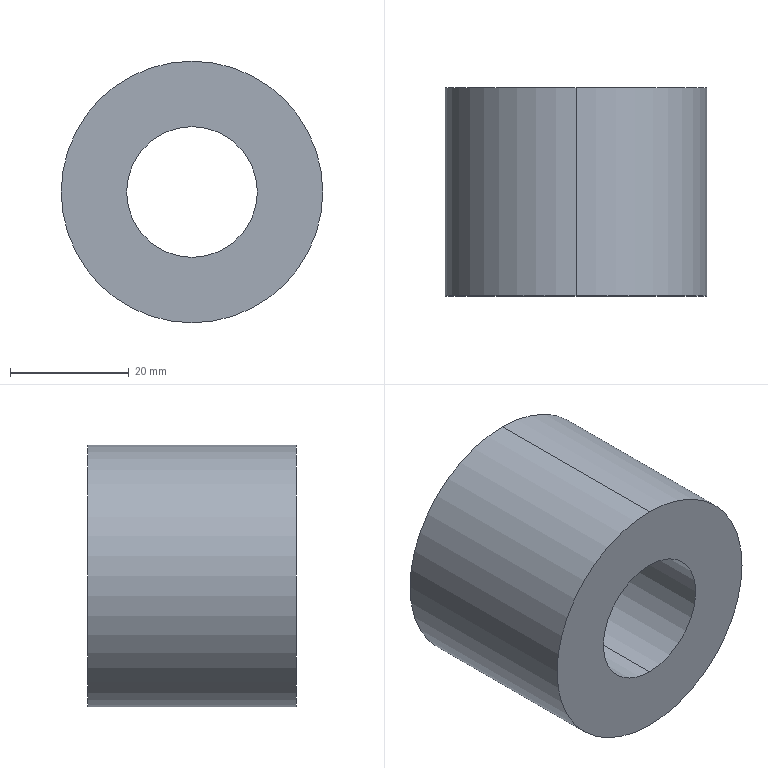Part | 1 solid | 6 faces | box 44 x 35 x 44 mm | volume 39914 mm3 | cylinder 4 | plane 2 | commonest cylinder face diameters 22 x2 44 x2
STEP:
#1=CARTESIAN_POINT('',(0.,0.,0.));
#2=DIRECTION('',(0.,0.,1.));
#3=DIRECTION('',(1.,0.,0.));
#4=AXIS2_PLACEMENT_3D('',#1,#2,#3);
#5=CARTESIAN_POINT('',(-359.028,244.5,-322.55));
#6=VERTEX_POINT('',#5);
#7=CARTESIAN_POINT('',(-359.028,244.5,-278.55));
#8=VERTEX_POINT('',#7);
#9=CARTESIAN_POINT('',(-359.028,244.5,-300.55));
#10=DIRECTION('',(0.,1.,0.));
#11=DIRECTION('',(0.,0.,-1.));
#12=AXIS2_PLACEMENT_3D('',#9,#10,#11);
#13=CIRCLE('',#12,22.);
#14=CARTESIAN_POINT('',(-359.028,244.5,-300.55));
#15=DIRECTION('',(0.,-1.,0.));
#16=DIRECTION('',(0.,0.,-1.));
#17=AXIS2_PLACEMENT_3D('',#14,#15,#16);
#18=PLANE('',#17);
#19=CARTESIAN_POINT('',(22.,0.));
#20=CARTESIAN_POINT('',(22.,-38.105));
#21=CARTESIAN_POINT('',(-11.,-19.053));
#22=CARTESIAN_POINT('',(-44.,0.));
#23=CARTESIAN_POINT('',(-11.,19.053));
#24=CARTESIAN_POINT('',(22.,38.105));
#25=CARTESIAN_POINT('',(22.,0.));
#26=(BOUNDED_CURVE()B_SPLINE_CURVE(2,(#19,#20,#21,#22,#23,#24,#25),.UNSPECIFIED.,.T.,.F.)B_SPLINE_CURVE_WITH_KNOTS((1,2,2,2,2,1),(-2.094,0.,2.094,4.189,6.283,8.378),.UNSPECIFIED.)CURVE()GEOMETRIC_REPRESENTATION_ITEM()RATIONAL_B_SPLINE_CURVE((1.,0.5,1.,0.5,1.,0.5,1.))REPRESENTATION_ITEM(''));
#27=(GEOMETRIC_REPRESENTATION_CONTEXT(2)PARAMETRIC_REPRESENTATION_CONTEXT()REPRESENTATION_CONTEXT('',''));
#28=DEFINITIONAL_REPRESENTATION('',(#26),#27);
#29=PCURVE('',#18,#28);
#30=CARTESIAN_POINT('',(-359.028,244.5,-300.55));
#31=DIRECTION('',(0.,-1.,0.));
#32=DIRECTION('',(1.,0.,0.));
#33=AXIS2_PLACEMENT_3D('',#30,#31,#32);
#34=CYLINDRICAL_SURFACE('',#33,22.);
#35=CARTESIAN_POINT('',(4.712,0.));
#36=DIRECTION('',(-1.,0.));
#37=VECTOR('',#36,1.);
#38=LINE('',#35,#37);
#39=(GEOMETRIC_REPRESENTATION_CONTEXT(2)PARAMETRIC_REPRESENTATION_CONTEXT()REPRESENTATION_CONTEXT('',''));
#40=DEFINITIONAL_REPRESENTATION('',(#38),#39);
#41=PCURVE('',#34,#40);
#42=SURFACE_CURVE('',#13,(#29,#41),.PCURVE_S1.);
#43=EDGE_CURVE('',#6,#8,#42,.T.);
#44=ORIENTED_EDGE('',*,*,#43,.T.);
#45=CARTESIAN_POINT('',(-359.028,244.5,-300.55));
#46=DIRECTION('',(0.,1.,0.));
#47=DIRECTION('',(0.,0.,-1.));
#48=AXIS2_PLACEMENT_3D('',#45,#46,#47);
#49=CIRCLE('',#48,22.);
#50=CARTESIAN_POINT('',(22.,0.));
#51=CARTESIAN_POINT('',(22.,-38.105));
#52=CARTESIAN_POINT('',(-11.,-19.053));
#53=CARTESIAN_POINT('',(-44.,0.));
#54=CARTESIAN_POINT('',(-11.,19.053));
#55=CARTESIAN_POINT('',(22.,38.105));
#56=CARTESIAN_POINT('',(22.,0.));
#57=(BOUNDED_CURVE()B_SPLINE_CURVE(2,(#50,#51,#52,#53,#54,#55,#56),.UNSPECIFIED.,.T.,.F.)B_SPLINE_CURVE_WITH_KNOTS((1,2,2,2,2,1),(-2.094,0.,2.094,4.189,6.283,8.378),.UNSPECIFIED.)CURVE()GEOMETRIC_REPRESENTATION_ITEM()RATIONAL_B_SPLINE_CURVE((1.,0.5,1.,0.5,1.,0.5,1.))REPRESENTATION_ITEM(''));
#58=(GEOMETRIC_REPRESENTATION_CONTEXT(2)PARAMETRIC_REPRESENTATION_CONTEXT()REPRESENTATION_CONTEXT('',''));
#59=DEFINITIONAL_REPRESENTATION('',(#57),#58);
#60=PCURVE('',#18,#59);
#61=CARTESIAN_POINT('',(-359.028,244.5,-300.55));
#62=DIRECTION('',(0.,-1.,0.));
#63=DIRECTION('',(-1.,0.,0.));
#64=AXIS2_PLACEMENT_3D('',#61,#62,#63);
#65=CYLINDRICAL_SURFACE('',#64,22.);
#66=CARTESIAN_POINT('',(7.854,0.));
#67=DIRECTION('',(-1.,0.));
#68=VECTOR('',#67,1.);
#69=LINE('',#66,#68);
#70=(GEOMETRIC_REPRESENTATION_CONTEXT(2)PARAMETRIC_REPRESENTATION_CONTEXT()REPRESENTATION_CONTEXT('',''));
#71=DEFINITIONAL_REPRESENTATION('',(#69),#70);
#72=PCURVE('',#65,#71);
#73=SURFACE_CURVE('',#49,(#60,#72),.PCURVE_S1.);
#74=EDGE_CURVE('',#8,#6,#73,.T.);
#75=ORIENTED_EDGE('',*,*,#74,.T.);
#76=EDGE_LOOP('',(#44,#75));
#77=FACE_BOUND('',#76,.T.);
#78=CARTESIAN_POINT('',(-359.028,244.5,-289.55));
#79=VERTEX_POINT('',#78);
#80=CARTESIAN_POINT('',(-359.028,244.5,-311.55));
#81=VERTEX_POINT('',#80);
#82=CARTESIAN_POINT('',(-359.028,244.5,-300.55));
#83=DIRECTION('',(0.,1.,0.));
#84=DIRECTION('',(0.,0.,-1.));
#85=AXIS2_PLACEMENT_3D('',#82,#83,#84);
#86=CIRCLE('',#85,11.);
#87=CARTESIAN_POINT('',(11.,0.));
#88=CARTESIAN_POINT('',(11.,-19.053));
#89=CARTESIAN_POINT('',(-5.5,-9.526));
#90=CARTESIAN_POINT('',(-22.,0.));
#91=CARTESIAN_POINT('',(-5.5,9.526));
#92=CARTESIAN_POINT('',(11.,19.053));
#93=CARTESIAN_POINT('',(11.,0.));
#94=(BOUNDED_CURVE()B_SPLINE_CURVE(2,(#87,#88,#89,#90,#91,#92,#93),.UNSPECIFIED.,.T.,.F.)B_SPLINE_CURVE_WITH_KNOTS((1,2,2,2,2,1),(-2.094,0.,2.094,4.189,6.283,8.378),.UNSPECIFIED.)CURVE()GEOMETRIC_REPRESENTATION_ITEM()RATIONAL_B_SPLINE_CURVE((1.,0.5,1.,0.5,1.,0.5,1.))REPRESENTATION_ITEM(''));
#95=(GEOMETRIC_REPRESENTATION_CONTEXT(2)PARAMETRIC_REPRESENTATION_CONTEXT()REPRESENTATION_CONTEXT('',''));
#96=DEFINITIONAL_REPRESENTATION('',(#94),#95);
#97=PCURVE('',#18,#96);
#98=CARTESIAN_POINT('',(-359.028,244.5,-300.55));
#99=DIRECTION('',(0.,-1.,0.));
#100=DIRECTION('',(-1.,0.,0.));
#101=AXIS2_PLACEMENT_3D('',#98,#99,#100);
#102=CYLINDRICAL_SURFACE('',#101,11.);
#103=CARTESIAN_POINT('',(7.854,0.));
#104=DIRECTION('',(-1.,0.));
#105=VECTOR('',#104,1.);
#106=LINE('',#103,#105);
#107=(GEOMETRIC_REPRESENTATION_CONTEXT(2)PARAMETRIC_REPRESENTATION_CONTEXT()REPRESENTATION_CONTEXT('',''));
#108=DEFINITIONAL_REPRESENTATION('',(#106),#107);
#109=PCURVE('',#102,#108);
#110=SURFACE_CURVE('',#86,(#97,#109),.PCURVE_S1.);
#111=EDGE_CURVE('',#79,#81,#110,.T.);
#112=ORIENTED_EDGE('',*,*,#111,.F.);
#113=CARTESIAN_POINT('',(-359.028,244.5,-300.55));
#114=DIRECTION('',(0.,1.,0.));
#115=DIRECTION('',(0.,0.,-1.));
#116=AXIS2_PLACEMENT_3D('',#113,#114,#115);
#117=CIRCLE('',#116,11.);
#118=CARTESIAN_POINT('',(11.,0.));
#119=CARTESIAN_POINT('',(11.,-19.053));
#120=CARTESIAN_POINT('',(-5.5,-9.526));
#121=CARTESIAN_POINT('',(-22.,0.));
#122=CARTESIAN_POINT('',(-5.5,9.526));
#123=CARTESIAN_POINT('',(11.,19.053));
#124=CARTESIAN_POINT('',(11.,0.));
#125=(BOUNDED_CURVE()B_SPLINE_CURVE(2,(#118,#119,#120,#121,#122,#123,#124),.UNSPECIFIED.,.T.,.F.)B_SPLINE_CURVE_WITH_KNOTS((1,2,2,2,2,1),(-2.094,0.,2.094,4.189,6.283,8.378),.UNSPECIFIED.)CURVE()GEOMETRIC_REPRESENTATION_ITEM()RATIONAL_B_SPLINE_CURVE((1.,0.5,1.,0.5,1.,0.5,1.))REPRESENTATION_ITEM(''));
#126=(GEOMETRIC_REPRESENTATION_CONTEXT(2)PARAMETRIC_REPRESENTATION_CONTEXT()REPRESENTATION_CONTEXT('',''));
#127=DEFINITIONAL_REPRESENTATION('',(#125),#126);
#128=PCURVE('',#18,#127);
#129=CARTESIAN_POINT('',(-359.028,244.5,-300.55));
#130=DIRECTION('',(0.,-1.,0.));
#131=DIRECTION('',(1.,0.,0.));
#132=AXIS2_PLACEMENT_3D('',#129,#130,#131);
#133=CYLINDRICAL_SURFACE('',#132,11.);
#134=CARTESIAN_POINT('',(4.712,0.));
#135=DIRECTION('',(-1.,0.));
#136=VECTOR('',#135,1.);
#137=LINE('',#134,#136);
#138=(GEOMETRIC_REPRESENTATION_CONTEXT(2)PARAMETRIC_REPRESENTATION_CONTEXT()REPRESENTATION_CONTEXT('',''));
#139=DEFINITIONAL_REPRESENTATION('',(#137),#138);
#140=PCURVE('',#133,#139);
#141=SURFACE_CURVE('',#117,(#128,#140),.PCURVE_S1.);
#142=EDGE_CURVE('',#81,#79,#141,.T.);
#143=ORIENTED_EDGE('',*,*,#142,.F.);
#144=EDGE_LOOP('',(#112,#143));
#145=FACE_BOUND('',#144,.T.);
#146=ADVANCED_FACE('',(#77,#145),#18,.F.);
#147=ORIENTED_EDGE('',*,*,#142,.F.);
#148=CARTESIAN_POINT('',(-359.028,209.5,-311.55));
#149=VERTEX_POINT('',#148);
#150=CARTESIAN_POINT('',(-359.028,244.5,-311.55));
#151=DIRECTION('',(0.,-1.,0.));
#152=VECTOR('',#151,1.);
#153=LINE('',#150,#152);
#154=CARTESIAN_POINT('',(4.712,0.));
#155=DIRECTION('',(0.,1.));
#156=VECTOR('',#155,1.);
#157=LINE('',#154,#156);
#158=(GEOMETRIC_REPRESENTATION_CONTEXT(2)PARAMETRIC_REPRESENTATION_CONTEXT()REPRESENTATION_CONTEXT('',''));
#159=DEFINITIONAL_REPRESENTATION('',(#157),#158);
#160=PCURVE('',#133,#159);
#161=CARTESIAN_POINT('',(1.571,0.));
#162=DIRECTION('',(0.,1.));
#163=VECTOR('',#162,1.);
#164=LINE('',#161,#163);
#165=(GEOMETRIC_REPRESENTATION_CONTEXT(2)PARAMETRIC_REPRESENTATION_CONTEXT()REPRESENTATION_CONTEXT('',''));
#166=DEFINITIONAL_REPRESENTATION('',(#164),#165);
#167=PCURVE('',#102,#166);
#168=SURFACE_CURVE('',#153,(#160,#167),.PCURVE_S1.);
#169=EDGE_CURVE('',#81,#149,#168,.T.);
#170=ORIENTED_EDGE('',*,*,#169,.T.);
#171=CARTESIAN_POINT('',(-359.028,209.5,-289.55));
#172=VERTEX_POINT('',#171);
#173=CARTESIAN_POINT('',(-359.028,209.5,-300.55));
#174=DIRECTION('',(0.,1.,0.));
#175=DIRECTION('',(0.,0.,-1.));
#176=AXIS2_PLACEMENT_3D('',#173,#174,#175);
#177=CIRCLE('',#176,11.);
#178=CARTESIAN_POINT('',(4.712,35.));
#179=DIRECTION('',(-1.,0.));
#180=VECTOR('',#179,1.);
#181=LINE('',#178,#180);
#182=(GEOMETRIC_REPRESENTATION_CONTEXT(2)PARAMETRIC_REPRESENTATION_CONTEXT()REPRESENTATION_CONTEXT('',''));
#183=DEFINITIONAL_REPRESENTATION('',(#181),#182);
#184=PCURVE('',#133,#183);
#185=CARTESIAN_POINT('',(-359.028,209.5,-300.55));
#186=DIRECTION('',(0.,-1.,0.));
#187=DIRECTION('',(0.,0.,-1.));
#188=AXIS2_PLACEMENT_3D('',#185,#186,#187);
#189=PLANE('',#188);
#190=CARTESIAN_POINT('',(11.,0.));
#191=CARTESIAN_POINT('',(11.,-19.053));
#192=CARTESIAN_POINT('',(-5.5,-9.526));
#193=CARTESIAN_POINT('',(-22.,0.));
#194=CARTESIAN_POINT('',(-5.5,9.526));
#195=CARTESIAN_POINT('',(11.,19.053));
#196=CARTESIAN_POINT('',(11.,0.));
#197=(BOUNDED_CURVE()B_SPLINE_CURVE(2,(#190,#191,#192,#193,#194,#195,#196),.UNSPECIFIED.,.T.,.F.)B_SPLINE_CURVE_WITH_KNOTS((1,2,2,2,2,1),(-2.094,0.,2.094,4.189,6.283,8.378),.UNSPECIFIED.)CURVE()GEOMETRIC_REPRESENTATION_ITEM()RATIONAL_B_SPLINE_CURVE((1.,0.5,1.,0.5,1.,0.5,1.))REPRESENTATION_ITEM(''));
#198=(GEOMETRIC_REPRESENTATION_CONTEXT(2)PARAMETRIC_REPRESENTATION_CONTEXT()REPRESENTATION_CONTEXT('',''));
#199=DEFINITIONAL_REPRESENTATION('',(#197),#198);
#200=PCURVE('',#189,#199);
#201=SURFACE_CURVE('',#177,(#184,#200),.PCURVE_S1.);
#202=EDGE_CURVE('',#149,#172,#201,.T.);
#203=ORIENTED_EDGE('',*,*,#202,.T.);
#204=CARTESIAN_POINT('',(-359.028,244.5,-289.55));
#205=DIRECTION('',(0.,-1.,0.));
#206=VECTOR('',#205,1.);
#207=LINE('',#204,#206);
#208=CARTESIAN_POINT('',(1.571,0.));
#209=DIRECTION('',(0.,1.));
#210=VECTOR('',#209,1.);
#211=LINE('',#208,#210);
#212=(GEOMETRIC_REPRESENTATION_CONTEXT(2)PARAMETRIC_REPRESENTATION_CONTEXT()REPRESENTATION_CONTEXT('',''));
#213=DEFINITIONAL_REPRESENTATION('',(#211),#212);
#214=PCURVE('',#133,#213);
#215=CARTESIAN_POINT('',(4.712,0.));
#216=DIRECTION('',(0.,1.));
#217=VECTOR('',#216,1.);
#218=LINE('',#215,#217);
#219=(GEOMETRIC_REPRESENTATION_CONTEXT(2)PARAMETRIC_REPRESENTATION_CONTEXT()REPRESENTATION_CONTEXT('',''));
#220=DEFINITIONAL_REPRESENTATION('',(#218),#219);
#221=PCURVE('',#102,#220);
#222=SURFACE_CURVE('',#207,(#214,#221),.PCURVE_S1.);
#223=EDGE_CURVE('',#79,#172,#222,.T.);
#224=ORIENTED_EDGE('',*,*,#223,.F.);
#225=EDGE_LOOP('',(#147,#170,#203,#224));
#226=FACE_BOUND('',#225,.F.);
#227=ADVANCED_FACE('',(#226),#133,.F.);
#228=CARTESIAN_POINT('',(-359.028,209.5,-278.55));
#229=VERTEX_POINT('',#228);
#230=CARTESIAN_POINT('',(-359.028,209.5,-322.55));
#231=VERTEX_POINT('',#230);
#232=CARTESIAN_POINT('',(-359.028,209.5,-300.55));
#233=DIRECTION('',(0.,1.,0.));
#234=DIRECTION('',(0.,0.,-1.));
#235=AXIS2_PLACEMENT_3D('',#232,#233,#234);
#236=CIRCLE('',#235,22.);
#237=CARTESIAN_POINT('',(22.,0.));
#238=CARTESIAN_POINT('',(22.,-38.105));
#239=CARTESIAN_POINT('',(-11.,-19.053));
#240=CARTESIAN_POINT('',(-44.,0.));
#241=CARTESIAN_POINT('',(-11.,19.053));
#242=CARTESIAN_POINT('',(22.,38.105));
#243=CARTESIAN_POINT('',(22.,0.));
#244=(BOUNDED_CURVE()B_SPLINE_CURVE(2,(#237,#238,#239,#240,#241,#242,#243),.UNSPECIFIED.,.T.,.F.)B_SPLINE_CURVE_WITH_KNOTS((1,2,2,2,2,1),(-2.094,0.,2.094,4.189,6.283,8.378),.UNSPECIFIED.)CURVE()GEOMETRIC_REPRESENTATION_ITEM()RATIONAL_B_SPLINE_CURVE((1.,0.5,1.,0.5,1.,0.5,1.))REPRESENTATION_ITEM(''));
#245=(GEOMETRIC_REPRESENTATION_CONTEXT(2)PARAMETRIC_REPRESENTATION_CONTEXT()REPRESENTATION_CONTEXT('',''));
#246=DEFINITIONAL_REPRESENTATION('',(#244),#245);
#247=PCURVE('',#189,#246);
#248=CARTESIAN_POINT('',(7.854,35.));
#249=DIRECTION('',(-1.,0.));
#250=VECTOR('',#249,1.);
#251=LINE('',#248,#250);
#252=(GEOMETRIC_REPRESENTATION_CONTEXT(2)PARAMETRIC_REPRESENTATION_CONTEXT()REPRESENTATION_CONTEXT('',''));
#253=DEFINITIONAL_REPRESENTATION('',(#251),#252);
#254=PCURVE('',#65,#253);
#255=SURFACE_CURVE('',#236,(#247,#254),.PCURVE_S1.);
#256=EDGE_CURVE('',#229,#231,#255,.T.);
#257=ORIENTED_EDGE('',*,*,#256,.F.);
#258=CARTESIAN_POINT('',(-359.028,209.5,-300.55));
#259=DIRECTION('',(0.,1.,0.));
#260=DIRECTION('',(0.,0.,-1.));
#261=AXIS2_PLACEMENT_3D('',#258,#259,#260);
#262=CIRCLE('',#261,22.);
#263=CARTESIAN_POINT('',(22.,0.));
#264=CARTESIAN_POINT('',(22.,-38.105));
#265=CARTESIAN_POINT('',(-11.,-19.053));
#266=CARTESIAN_POINT('',(-44.,0.));
#267=CARTESIAN_POINT('',(-11.,19.053));
#268=CARTESIAN_POINT('',(22.,38.105));
#269=CARTESIAN_POINT('',(22.,0.));
#270=(BOUNDED_CURVE()B_SPLINE_CURVE(2,(#263,#264,#265,#266,#267,#268,#269),.UNSPECIFIED.,.T.,.F.)B_SPLINE_CURVE_WITH_KNOTS((1,2,2,2,2,1),(-2.094,0.,2.094,4.189,6.283,8.378),.UNSPECIFIED.)CURVE()GEOMETRIC_REPRESENTATION_ITEM()RATIONAL_B_SPLINE_CURVE((1.,0.5,1.,0.5,1.,0.5,1.))REPRESENTATION_ITEM(''));
#271=(GEOMETRIC_REPRESENTATION_CONTEXT(2)PARAMETRIC_REPRESENTATION_CONTEXT()REPRESENTATION_CONTEXT('',''));
#272=DEFINITIONAL_REPRESENTATION('',(#270),#271);
#273=PCURVE('',#189,#272);
#274=CARTESIAN_POINT('',(4.712,35.));
#275=DIRECTION('',(-1.,0.));
#276=VECTOR('',#275,1.);
#277=LINE('',#274,#276);
#278=(GEOMETRIC_REPRESENTATION_CONTEXT(2)PARAMETRIC_REPRESENTATION_CONTEXT()REPRESENTATION_CONTEXT('',''));
#279=DEFINITIONAL_REPRESENTATION('',(#277),#278);
#280=PCURVE('',#34,#279);
#281=SURFACE_CURVE('',#262,(#273,#280),.PCURVE_S1.);
#282=EDGE_CURVE('',#231,#229,#281,.T.);
#283=ORIENTED_EDGE('',*,*,#282,.F.);
#284=EDGE_LOOP('',(#257,#283));
#285=FACE_BOUND('',#284,.T.);
#286=ORIENTED_EDGE('',*,*,#202,.T.);
#287=CARTESIAN_POINT('',(-359.028,209.5,-300.55));
#288=DIRECTION('',(0.,1.,0.));
#289=DIRECTION('',(0.,0.,-1.));
#290=AXIS2_PLACEMENT_3D('',#287,#288,#289);
#291=CIRCLE('',#290,11.);
#292=CARTESIAN_POINT('',(11.,0.));
#293=CARTESIAN_POINT('',(11.,-19.053));
#294=CARTESIAN_POINT('',(-5.5,-9.526));
#295=CARTESIAN_POINT('',(-22.,0.));
#296=CARTESIAN_POINT('',(-5.5,9.526));
#297=CARTESIAN_POINT('',(11.,19.053));
#298=CARTESIAN_POINT('',(11.,0.));
#299=(BOUNDED_CURVE()B_SPLINE_CURVE(2,(#292,#293,#294,#295,#296,#297,#298),.UNSPECIFIED.,.T.,.F.)B_SPLINE_CURVE_WITH_KNOTS((1,2,2,2,2,1),(-2.094,0.,2.094,4.189,6.283,8.378),.UNSPECIFIED.)CURVE()GEOMETRIC_REPRESENTATION_ITEM()RATIONAL_B_SPLINE_CURVE((1.,0.5,1.,0.5,1.,0.5,1.))REPRESENTATION_ITEM(''));
#300=(GEOMETRIC_REPRESENTATION_CONTEXT(2)PARAMETRIC_REPRESENTATION_CONTEXT()REPRESENTATION_CONTEXT('',''));
#301=DEFINITIONAL_REPRESENTATION('',(#299),#300);
#302=PCURVE('',#189,#301);
#303=CARTESIAN_POINT('',(7.854,35.));
#304=DIRECTION('',(-1.,0.));
#305=VECTOR('',#304,1.);
#306=LINE('',#303,#305);
#307=(GEOMETRIC_REPRESENTATION_CONTEXT(2)PARAMETRIC_REPRESENTATION_CONTEXT()REPRESENTATION_CONTEXT('',''));
#308=DEFINITIONAL_REPRESENTATION('',(#306),#307);
#309=PCURVE('',#102,#308);
#310=SURFACE_CURVE('',#291,(#302,#309),.PCURVE_S1.);
#311=EDGE_CURVE('',#172,#149,#310,.T.);
#312=ORIENTED_EDGE('',*,*,#311,.T.);
#313=EDGE_LOOP('',(#286,#312));
#314=FACE_BOUND('',#313,.T.);
#315=ADVANCED_FACE('',(#285,#314),#189,.T.);
#316=CARTESIAN_POINT('',(-359.028,244.5,-278.55));
#317=DIRECTION('',(0.,-1.,0.));
#318=VECTOR('',#317,1.);
#319=LINE('',#316,#318);
#320=CARTESIAN_POINT('',(1.571,0.));
#321=DIRECTION('',(0.,1.));
#322=VECTOR('',#321,1.);
#323=LINE('',#320,#322);
#324=(GEOMETRIC_REPRESENTATION_CONTEXT(2)PARAMETRIC_REPRESENTATION_CONTEXT()REPRESENTATION_CONTEXT('',''));
#325=DEFINITIONAL_REPRESENTATION('',(#323),#324);
#326=PCURVE('',#34,#325);
#327=CARTESIAN_POINT('',(4.712,0.));
#328=DIRECTION('',(0.,1.));
#329=VECTOR('',#328,1.);
#330=LINE('',#327,#329);
#331=(GEOMETRIC_REPRESENTATION_CONTEXT(2)PARAMETRIC_REPRESENTATION_CONTEXT()REPRESENTATION_CONTEXT('',''));
#332=DEFINITIONAL_REPRESENTATION('',(#330),#331);
#333=PCURVE('',#65,#332);
#334=SURFACE_CURVE('',#319,(#326,#333),.PCURVE_S1.);
#335=EDGE_CURVE('',#8,#229,#334,.T.);
#336=ORIENTED_EDGE('',*,*,#335,.F.);
#337=ORIENTED_EDGE('',*,*,#43,.F.);
#338=CARTESIAN_POINT('',(-359.028,244.5,-322.55));
#339=DIRECTION('',(0.,-1.,0.));
#340=VECTOR('',#339,1.);
#341=LINE('',#338,#340);
#342=CARTESIAN_POINT('',(4.712,0.));
#343=DIRECTION('',(0.,1.));
#344=VECTOR('',#343,1.);
#345=LINE('',#342,#344);
#346=(GEOMETRIC_REPRESENTATION_CONTEXT(2)PARAMETRIC_REPRESENTATION_CONTEXT()REPRESENTATION_CONTEXT('',''));
#347=DEFINITIONAL_REPRESENTATION('',(#345),#346);
#348=PCURVE('',#34,#347);
#349=CARTESIAN_POINT('',(1.571,0.));
#350=DIRECTION('',(0.,1.));
#351=VECTOR('',#350,1.);
#352=LINE('',#349,#351);
#353=(GEOMETRIC_REPRESENTATION_CONTEXT(2)PARAMETRIC_REPRESENTATION_CONTEXT()REPRESENTATION_CONTEXT('',''));
#354=DEFINITIONAL_REPRESENTATION('',(#352),#353);
#355=PCURVE('',#65,#354);
#356=SURFACE_CURVE('',#341,(#348,#355),.PCURVE_S1.);
#357=EDGE_CURVE('',#6,#231,#356,.T.);
#358=ORIENTED_EDGE('',*,*,#357,.T.);
#359=ORIENTED_EDGE('',*,*,#282,.T.);
#360=EDGE_LOOP('',(#336,#337,#358,#359));
#361=FACE_BOUND('',#360,.T.);
#362=ADVANCED_FACE('',(#361),#34,.T.);
#363=ORIENTED_EDGE('',*,*,#311,.T.);
#364=ORIENTED_EDGE('',*,*,#169,.F.);
#365=ORIENTED_EDGE('',*,*,#111,.F.);
#366=ORIENTED_EDGE('',*,*,#223,.T.);
#367=EDGE_LOOP('',(#363,#364,#365,#366));
#368=FACE_BOUND('',#367,.F.);
#369=ADVANCED_FACE('',(#368),#102,.F.);
#370=ORIENTED_EDGE('',*,*,#335,.T.);
#371=ORIENTED_EDGE('',*,*,#256,.T.);
#372=ORIENTED_EDGE('',*,*,#357,.F.);
#373=ORIENTED_EDGE('',*,*,#74,.F.);
#374=EDGE_LOOP('',(#370,#371,#372,#373));
#375=FACE_BOUND('',#374,.T.);
#376=ADVANCED_FACE('',(#375),#65,.T.);
#377=CLOSED_SHELL('',(#146,#227,#315,#362,#369,#376));
#378=MANIFOLD_SOLID_BREP('',#377);
#379=(LENGTH_UNIT()NAMED_UNIT(*)SI_UNIT(.MILLI.,.METRE.));
#380=UNCERTAINTY_MEASURE_WITH_UNIT(LENGTH_MEASURE(0.0000001),#379,'','');
#381=(NAMED_UNIT(*)PLANE_ANGLE_UNIT()SI_UNIT($,.RADIAN.));
#382=(NAMED_UNIT(*)SI_UNIT($,.STERADIAN.)SOLID_ANGLE_UNIT());
#383=(GEOMETRIC_REPRESENTATION_CONTEXT(3)GLOBAL_UNCERTAINTY_ASSIGNED_CONTEXT((#380))GLOBAL_UNIT_ASSIGNED_CONTEXT((#379,#381,#382))REPRESENTATION_CONTEXT('',''));
#384=ADVANCED_BREP_SHAPE_REPRESENTATION('',(#4,#378),#383);